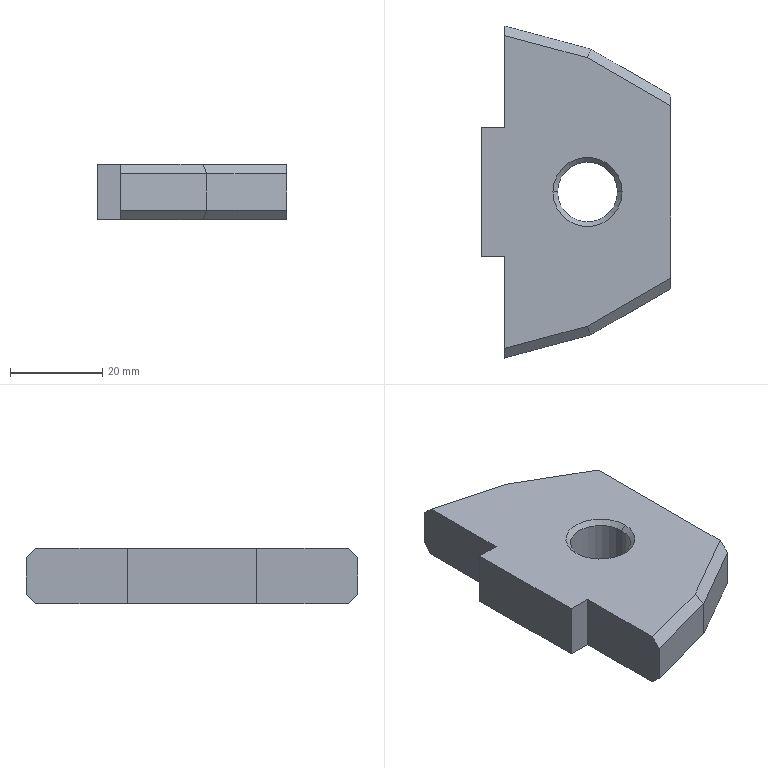Part | SolidWorks | features Chamfer 2, Extrusion 1 | 1 solid | 26 faces | box 41 x 72 x 12 mm | volume 25554 mm3 | plane 20 | cone 4 | cylinder 2 | commonest cylinder face diameters 13 x2
STEP:
#1=CARTESIAN_POINT('',(-6.5,0.,5.));
#2=VERTEX_POINT('',#1);
#3=CARTESIAN_POINT('',(6.5,0.,5.));
#4=VERTEX_POINT('',#3);
#5=CARTESIAN_POINT('',(0.,0.,5.));
#6=DIRECTION('',(0.,0.,1.));
#7=DIRECTION('',(-1.,0.,0.));
#8=AXIS2_PLACEMENT_3D('',#5,#6,#7);
#9=CIRCLE('',#8,6.5);
#10=EDGE_CURVE('',#2,#4,#9,.T.);
#11=ORIENTED_EDGE('',*,*,#10,.F.);
#12=CARTESIAN_POINT('',(-7.5,0.,6.));
#13=VERTEX_POINT('',#12);
#14=CARTESIAN_POINT('',(-7.5,0.,6.));
#15=DIRECTION('',(-0.7071,0.,0.7071));
#16=VECTOR('',#15,1000.);
#17=LINE('',#14,#16);
#18=EDGE_CURVE('',#2,#13,#17,.T.);
#19=ORIENTED_EDGE('',*,*,#18,.T.);
#20=CARTESIAN_POINT('',(7.5,0.,6.));
#21=VERTEX_POINT('',#20);
#22=CARTESIAN_POINT('',(0.,0.,6.));
#23=DIRECTION('',(0.,0.,-1.));
#24=DIRECTION('',(-1.,0.,0.));
#25=AXIS2_PLACEMENT_3D('',#22,#23,#24);
#26=CIRCLE('',#25,7.5);
#27=EDGE_CURVE('',#21,#13,#26,.T.);
#28=ORIENTED_EDGE('',*,*,#27,.F.);
#29=CARTESIAN_POINT('',(7.5,0.,6.));
#30=DIRECTION('',(0.7071,0.,0.7071));
#31=VECTOR('',#30,1000.);
#32=LINE('',#29,#31);
#33=EDGE_CURVE('',#4,#21,#32,.T.);
#34=ORIENTED_EDGE('',*,*,#33,.F.);
#35=EDGE_LOOP('',(#11,#19,#28,#34));
#36=FACE_OUTER_BOUND('',#35,.T.);
#37=CARTESIAN_POINT('',(0.,0.,6.));
#38=DIRECTION('',(0.,0.,1.));
#39=DIRECTION('',(1.,0.,0.));
#40=AXIS2_PLACEMENT_3D('',#37,#38,#39);
#41=CONICAL_SURFACE('',#40,7.5,0.7854);
#42=ADVANCED_FACE('',(#36),#41,.F.);
#43=CARTESIAN_POINT('',(6.5,0.,-5.));
#44=VERTEX_POINT('',#43);
#45=CARTESIAN_POINT('',(-6.5,0.,-5.));
#46=VERTEX_POINT('',#45);
#47=CARTESIAN_POINT('',(0.,0.,-5.));
#48=DIRECTION('',(0.,0.,-1.));
#49=DIRECTION('',(-1.,0.,0.));
#50=AXIS2_PLACEMENT_3D('',#47,#48,#49);
#51=CIRCLE('',#50,6.5);
#52=EDGE_CURVE('',#44,#46,#51,.T.);
#53=ORIENTED_EDGE('',*,*,#52,.F.);
#54=CARTESIAN_POINT('',(7.5,0.,-6.));
#55=VERTEX_POINT('',#54);
#56=CARTESIAN_POINT('',(6.5,0.,-5.));
#57=DIRECTION('',(0.7071,0.,-0.7071));
#58=VECTOR('',#57,1000.);
#59=LINE('',#56,#58);
#60=EDGE_CURVE('',#44,#55,#59,.T.);
#61=ORIENTED_EDGE('',*,*,#60,.T.);
#62=CARTESIAN_POINT('',(-7.5,0.,-6.));
#63=VERTEX_POINT('',#62);
#64=CARTESIAN_POINT('',(0.,0.,-6.));
#65=DIRECTION('',(0.,0.,1.));
#66=DIRECTION('',(-1.,0.,0.));
#67=AXIS2_PLACEMENT_3D('',#64,#65,#66);
#68=CIRCLE('',#67,7.5);
#69=EDGE_CURVE('',#63,#55,#68,.T.);
#70=ORIENTED_EDGE('',*,*,#69,.F.);
#71=CARTESIAN_POINT('',(-6.5,0.,-5.));
#72=DIRECTION('',(-0.7071,0.,-0.7071));
#73=VECTOR('',#72,1000.);
#74=LINE('',#71,#73);
#75=EDGE_CURVE('',#46,#63,#74,.T.);
#76=ORIENTED_EDGE('',*,*,#75,.F.);
#77=EDGE_LOOP('',(#53,#61,#70,#76));
#78=FACE_OUTER_BOUND('',#77,.T.);
#79=CARTESIAN_POINT('',(0.,0.,-5.));
#80=DIRECTION('',(0.,0.,-1.));
#81=DIRECTION('',(-1.,0.,0.));
#82=AXIS2_PLACEMENT_3D('',#79,#80,#81);
#83=CONICAL_SURFACE('',#82,6.5,0.7854);
#84=ADVANCED_FACE('',(#78),#83,.F.);
#85=ORIENTED_EDGE('',*,*,#10,.T.);
#86=CARTESIAN_POINT('',(6.5,0.,6.));
#87=DIRECTION('',(0.,0.,-1.));
#88=VECTOR('',#87,1000.);
#89=LINE('',#86,#88);
#90=EDGE_CURVE('',#4,#44,#89,.T.);
#91=ORIENTED_EDGE('',*,*,#90,.T.);
#92=ORIENTED_EDGE('',*,*,#52,.T.);
#93=CARTESIAN_POINT('',(-6.5,0.,6.));
#94=DIRECTION('',(0.,0.,-1.));
#95=VECTOR('',#94,1000.);
#96=LINE('',#93,#95);
#97=EDGE_CURVE('',#2,#46,#96,.T.);
#98=ORIENTED_EDGE('',*,*,#97,.F.);
#99=EDGE_LOOP('',(#85,#91,#92,#98));
#100=FACE_OUTER_BOUND('',#99,.T.);
#101=CARTESIAN_POINT('',(0.,0.,6.));
#102=DIRECTION('',(0.,0.,-1.));
#103=DIRECTION('',(-1.,0.,0.));
#104=AXIS2_PLACEMENT_3D('',#101,#102,#103);
#105=CYLINDRICAL_SURFACE('',#104,6.5);
#106=ADVANCED_FACE('',(#100),#105,.F.);
#107=CARTESIAN_POINT('',(-18.,36.,4.));
#108=VERTEX_POINT('',#107);
#109=CARTESIAN_POINT('',(-18.,36.,-4.));
#110=VERTEX_POINT('',#109);
#111=CARTESIAN_POINT('',(-18.,36.,6.));
#112=DIRECTION('',(0.,0.,-1.));
#113=VECTOR('',#112,1000.);
#114=LINE('',#111,#113);
#115=EDGE_CURVE('',#108,#110,#114,.T.);
#116=ORIENTED_EDGE('',*,*,#115,.T.);
#117=CARTESIAN_POINT('',(-18.,33.929,-6.));
#118=VERTEX_POINT('',#117);
#119=CARTESIAN_POINT('',(-18.,29.616,-10.167));
#120=DIRECTION('',(0.,-0.7193,-0.6947));
#121=VECTOR('',#120,1000.);
#122=LINE('',#119,#121);
#123=EDGE_CURVE('',#110,#118,#122,.T.);
#124=ORIENTED_EDGE('',*,*,#123,.T.);
#125=CARTESIAN_POINT('',(-18.,14.,-6.));
#126=VERTEX_POINT('',#125);
#127=CARTESIAN_POINT('',(-18.,14.,-6.));
#128=DIRECTION('',(0.,1.,0.));
#129=VECTOR('',#128,1000.);
#130=LINE('',#127,#129);
#131=EDGE_CURVE('',#126,#118,#130,.T.);
#132=ORIENTED_EDGE('',*,*,#131,.F.);
#133=CARTESIAN_POINT('',(-18.,14.,6.));
#134=VERTEX_POINT('',#133);
#135=CARTESIAN_POINT('',(-18.,14.,6.));
#136=DIRECTION('',(0.,0.,-1.));
#137=VECTOR('',#136,1000.);
#138=LINE('',#135,#137);
#139=EDGE_CURVE('',#134,#126,#138,.T.);
#140=ORIENTED_EDGE('',*,*,#139,.F.);
#141=CARTESIAN_POINT('',(-18.,33.929,6.));
#142=VERTEX_POINT('',#141);
#143=CARTESIAN_POINT('',(-18.,14.,6.));
#144=DIRECTION('',(0.,1.,0.));
#145=VECTOR('',#144,1000.);
#146=LINE('',#143,#145);
#147=EDGE_CURVE('',#134,#142,#146,.T.);
#148=ORIENTED_EDGE('',*,*,#147,.T.);
#149=CARTESIAN_POINT('',(-18.,23.619,15.959));
#150=DIRECTION('',(0.,0.7193,-0.6947));
#151=VECTOR('',#150,1000.);
#152=LINE('',#149,#151);
#153=EDGE_CURVE('',#142,#108,#152,.T.);
#154=ORIENTED_EDGE('',*,*,#153,.T.);
#155=EDGE_LOOP('',(#116,#124,#132,#140,#148,#154));
#156=FACE_OUTER_BOUND('',#155,.T.);
#157=CARTESIAN_POINT('',(-18.,14.,6.));
#158=DIRECTION('',(-1.,0.,0.));
#159=DIRECTION('',(0.,0.,1.));
#160=AXIS2_PLACEMENT_3D('',#157,#158,#159);
#161=PLANE('',#160);
#162=ADVANCED_FACE('',(#156),#161,.T.);
#163=CARTESIAN_POINT('',(-23.,14.,-6.));
#164=VERTEX_POINT('',#163);
#165=CARTESIAN_POINT('',(-23.,14.,-6.));
#166=DIRECTION('',(1.,0.,0.));
#167=VECTOR('',#166,1000.);
#168=LINE('',#165,#167);
#169=EDGE_CURVE('',#164,#126,#168,.T.);
#170=ORIENTED_EDGE('',*,*,#169,.F.);
#171=CARTESIAN_POINT('',(-23.,14.,6.));
#172=VERTEX_POINT('',#171);
#173=CARTESIAN_POINT('',(-23.,14.,6.));
#174=DIRECTION('',(0.,0.,-1.));
#175=VECTOR('',#174,1000.);
#176=LINE('',#173,#175);
#177=EDGE_CURVE('',#172,#164,#176,.T.);
#178=ORIENTED_EDGE('',*,*,#177,.F.);
#179=CARTESIAN_POINT('',(-23.,14.,6.));
#180=DIRECTION('',(1.,0.,0.));
#181=VECTOR('',#180,1000.);
#182=LINE('',#179,#181);
#183=EDGE_CURVE('',#172,#134,#182,.T.);
#184=ORIENTED_EDGE('',*,*,#183,.T.);
#185=ORIENTED_EDGE('',*,*,#139,.T.);
#186=EDGE_LOOP('',(#170,#178,#184,#185));
#187=FACE_OUTER_BOUND('',#186,.T.);
#188=CARTESIAN_POINT('',(-23.,14.,6.));
#189=DIRECTION('',(0.,1.,0.));
#190=DIRECTION('',(0.,0.,1.));
#191=AXIS2_PLACEMENT_3D('',#188,#189,#190);
#192=PLANE('',#191);
#193=ADVANCED_FACE('',(#187),#192,.T.);
#194=CARTESIAN_POINT('',(-23.,-14.,-6.));
#195=VERTEX_POINT('',#194);
#196=CARTESIAN_POINT('',(-23.,-14.,-6.));
#197=DIRECTION('',(0.,1.,0.));
#198=VECTOR('',#197,1000.);
#199=LINE('',#196,#198);
#200=EDGE_CURVE('',#195,#164,#199,.T.);
#201=ORIENTED_EDGE('',*,*,#200,.F.);
#202=CARTESIAN_POINT('',(-23.,-14.,6.));
#203=VERTEX_POINT('',#202);
#204=CARTESIAN_POINT('',(-23.,-14.,6.));
#205=DIRECTION('',(0.,0.,-1.));
#206=VECTOR('',#205,1000.);
#207=LINE('',#204,#206);
#208=EDGE_CURVE('',#203,#195,#207,.T.);
#209=ORIENTED_EDGE('',*,*,#208,.F.);
#210=CARTESIAN_POINT('',(-23.,-14.,6.));
#211=DIRECTION('',(0.,1.,0.));
#212=VECTOR('',#211,1000.);
#213=LINE('',#210,#212);
#214=EDGE_CURVE('',#203,#172,#213,.T.);
#215=ORIENTED_EDGE('',*,*,#214,.T.);
#216=ORIENTED_EDGE('',*,*,#177,.T.);
#217=EDGE_LOOP('',(#201,#209,#215,#216));
#218=FACE_OUTER_BOUND('',#217,.T.);
#219=CARTESIAN_POINT('',(-23.,-14.,6.));
#220=DIRECTION('',(-1.,0.,0.));
#221=DIRECTION('',(0.,0.,1.));
#222=AXIS2_PLACEMENT_3D('',#219,#220,#221);
#223=PLANE('',#222);
#224=ADVANCED_FACE('',(#218),#223,.T.);
#225=CARTESIAN_POINT('',(-18.,-14.,-6.));
#226=VERTEX_POINT('',#225);
#227=CARTESIAN_POINT('',(-23.,-14.,-6.));
#228=DIRECTION('',(1.,0.,0.));
#229=VECTOR('',#228,1000.);
#230=LINE('',#227,#229);
#231=EDGE_CURVE('',#195,#226,#230,.T.);
#232=ORIENTED_EDGE('',*,*,#231,.T.);
#233=CARTESIAN_POINT('',(-18.,-14.,6.));
#234=VERTEX_POINT('',#233);
#235=CARTESIAN_POINT('',(-18.,-14.,6.));
#236=DIRECTION('',(0.,0.,-1.));
#237=VECTOR('',#236,1000.);
#238=LINE('',#235,#237);
#239=EDGE_CURVE('',#234,#226,#238,.T.);
#240=ORIENTED_EDGE('',*,*,#239,.F.);
#241=CARTESIAN_POINT('',(-23.,-14.,6.));
#242=DIRECTION('',(1.,0.,0.));
#243=VECTOR('',#242,1000.);
#244=LINE('',#241,#243);
#245=EDGE_CURVE('',#203,#234,#244,.T.);
#246=ORIENTED_EDGE('',*,*,#245,.F.);
#247=ORIENTED_EDGE('',*,*,#208,.T.);
#248=EDGE_LOOP('',(#232,#240,#246,#247));
#249=FACE_OUTER_BOUND('',#248,.T.);
#250=CARTESIAN_POINT('',(-23.,-14.,6.));
#251=DIRECTION('',(0.,1.,0.));
#252=DIRECTION('',(0.,0.,1.));
#253=AXIS2_PLACEMENT_3D('',#250,#251,#252);
#254=PLANE('',#253);
#255=ADVANCED_FACE('',(#249),#254,.F.);
#256=CARTESIAN_POINT('',(-18.,-33.929,-6.));
#257=VERTEX_POINT('',#256);
#258=CARTESIAN_POINT('',(-18.,-14.,-6.));
#259=DIRECTION('',(0.,-1.,0.));
#260=VECTOR('',#259,1000.);
#261=LINE('',#258,#260);
#262=EDGE_CURVE('',#226,#257,#261,.T.);
#263=ORIENTED_EDGE('',*,*,#262,.T.);
#264=CARTESIAN_POINT('',(-18.,-36.,-4.));
#265=VERTEX_POINT('',#264);
#266=CARTESIAN_POINT('',(-18.,-36.,-4.));
#267=DIRECTION('',(0.,-0.7193,0.6947));
#268=VECTOR('',#267,1000.);
#269=LINE('',#266,#268);
#270=EDGE_CURVE('',#257,#265,#269,.T.);
#271=ORIENTED_EDGE('',*,*,#270,.T.);
#272=CARTESIAN_POINT('',(-18.,-36.,4.));
#273=VERTEX_POINT('',#272);
#274=CARTESIAN_POINT('',(-18.,-36.,6.));
#275=DIRECTION('',(0.,0.,-1.));
#276=VECTOR('',#275,1000.);
#277=LINE('',#274,#276);
#278=EDGE_CURVE('',#273,#265,#277,.T.);
#279=ORIENTED_EDGE('',*,*,#278,.F.);
#280=CARTESIAN_POINT('',(-18.,-33.929,6.));
#281=VERTEX_POINT('',#280);
#282=CARTESIAN_POINT('',(-18.,-30.426,9.384));
#283=DIRECTION('',(0.,0.7193,0.6947));
#284=VECTOR('',#283,1000.);
#285=LINE('',#282,#284);
#286=EDGE_CURVE('',#273,#281,#285,.T.);
#287=ORIENTED_EDGE('',*,*,#286,.T.);
#288=CARTESIAN_POINT('',(-18.,-14.,6.));
#289=DIRECTION('',(0.,-1.,0.));
#290=VECTOR('',#289,1000.);
#291=LINE('',#288,#290);
#292=EDGE_CURVE('',#234,#281,#291,.T.);
#293=ORIENTED_EDGE('',*,*,#292,.F.);
#294=ORIENTED_EDGE('',*,*,#239,.T.);
#295=EDGE_LOOP('',(#263,#271,#279,#287,#293,#294));
#296=FACE_OUTER_BOUND('',#295,.T.);
#297=CARTESIAN_POINT('',(-18.,-14.,6.));
#298=DIRECTION('',(1.,0.,0.));
#299=DIRECTION('',(0.,1.,0.));
#300=AXIS2_PLACEMENT_3D('',#297,#298,#299);
#301=PLANE('',#300);
#302=ADVANCED_FACE('',(#296),#301,.F.);
#303=ORIENTED_EDGE('',*,*,#278,.T.);
#304=CARTESIAN_POINT('',(0.6962,-30.99,-4.));
#305=VERTEX_POINT('',#304);
#306=CARTESIAN_POINT('',(0.6962,-30.99,-4.));
#307=DIRECTION('',(0.9659,0.2588,0.));
#308=VECTOR('',#307,1000.);
#309=LINE('',#306,#308);
#310=EDGE_CURVE('',#265,#305,#309,.T.);
#311=ORIENTED_EDGE('',*,*,#310,.T.);
#312=CARTESIAN_POINT('',(0.6962,-30.99,4.));
#313=VERTEX_POINT('',#312);
#314=CARTESIAN_POINT('',(0.6962,-30.99,6.));
#315=DIRECTION('',(0.,0.,-1.));
#316=VECTOR('',#315,1000.);
#317=LINE('',#314,#316);
#318=EDGE_CURVE('',#313,#305,#317,.T.);
#319=ORIENTED_EDGE('',*,*,#318,.F.);
#320=CARTESIAN_POINT('',(-18.,-36.,4.));
#321=DIRECTION('',(-0.9659,-0.2588,0.));
#322=VECTOR('',#321,1000.);
#323=LINE('',#320,#322);
#324=EDGE_CURVE('',#313,#273,#323,.T.);
#325=ORIENTED_EDGE('',*,*,#324,.T.);
#326=EDGE_LOOP('',(#303,#311,#319,#325));
#327=FACE_OUTER_BOUND('',#326,.T.);
#328=CARTESIAN_POINT('',(-18.,-36.,6.));
#329=DIRECTION('',(-0.2588,0.9659,0.));
#330=DIRECTION('',(-0.9659,-0.2588,0.));
#331=AXIS2_PLACEMENT_3D('',#328,#329,#330);
#332=PLANE('',#331);
#333=ADVANCED_FACE('',(#327),#332,.F.);
#334=ORIENTED_EDGE('',*,*,#318,.T.);
#335=CARTESIAN_POINT('',(18.,-21.,-4.));
#336=VERTEX_POINT('',#335);
#337=CARTESIAN_POINT('',(18.,-21.,-4.));
#338=DIRECTION('',(0.866,0.5,0.));
#339=VECTOR('',#338,1000.);
#340=LINE('',#337,#339);
#341=EDGE_CURVE('',#305,#336,#340,.T.);
#342=ORIENTED_EDGE('',*,*,#341,.T.);
#343=CARTESIAN_POINT('',(18.,-21.,4.));
#344=VERTEX_POINT('',#343);
#345=CARTESIAN_POINT('',(18.,-21.,6.));
#346=DIRECTION('',(0.,0.,-1.));
#347=VECTOR('',#346,1000.);
#348=LINE('',#345,#347);
#349=EDGE_CURVE('',#344,#336,#348,.T.);
#350=ORIENTED_EDGE('',*,*,#349,.F.);
#351=CARTESIAN_POINT('',(0.6962,-30.99,4.));
#352=DIRECTION('',(-0.866,-0.5,0.));
#353=VECTOR('',#352,1000.);
#354=LINE('',#351,#353);
#355=EDGE_CURVE('',#344,#313,#354,.T.);
#356=ORIENTED_EDGE('',*,*,#355,.T.);
#357=EDGE_LOOP('',(#334,#342,#350,#356));
#358=FACE_OUTER_BOUND('',#357,.T.);
#359=CARTESIAN_POINT('',(0.6962,-30.99,6.));
#360=DIRECTION('',(-0.5,0.866,0.));
#361=DIRECTION('',(-0.866,-0.5,0.));
#362=AXIS2_PLACEMENT_3D('',#359,#360,#361);
#363=PLANE('',#362);
#364=ADVANCED_FACE('',(#358),#363,.F.);
#365=ORIENTED_EDGE('',*,*,#349,.T.);
#366=CARTESIAN_POINT('',(18.,-18.691,-6.));
#367=VERTEX_POINT('',#366);
#368=CARTESIAN_POINT('',(18.,-1.949,-20.499));
#369=DIRECTION('',(0.,0.7559,-0.6547));
#370=VECTOR('',#369,1000.);
#371=LINE('',#368,#370);
#372=EDGE_CURVE('',#336,#367,#371,.T.);
#373=ORIENTED_EDGE('',*,*,#372,.T.);
#374=CARTESIAN_POINT('',(18.,18.691,-6.));
#375=VERTEX_POINT('',#374);
#376=CARTESIAN_POINT('',(18.,21.,-6.));
#377=DIRECTION('',(0.,-1.,0.));
#378=VECTOR('',#377,1000.);
#379=LINE('',#376,#378);
#380=EDGE_CURVE('',#375,#367,#379,.T.);
#381=ORIENTED_EDGE('',*,*,#380,.F.);
#382=CARTESIAN_POINT('',(18.,21.,-4.));
#383=VERTEX_POINT('',#382);
#384=CARTESIAN_POINT('',(18.,25.949,0.2857));
#385=DIRECTION('',(0.,0.7559,0.6547));
#386=VECTOR('',#385,1000.);
#387=LINE('',#384,#386);
#388=EDGE_CURVE('',#375,#383,#387,.T.);
#389=ORIENTED_EDGE('',*,*,#388,.T.);
#390=CARTESIAN_POINT('',(18.,21.,4.));
#391=VERTEX_POINT('',#390);
#392=CARTESIAN_POINT('',(18.,21.,6.));
#393=DIRECTION('',(0.,0.,-1.));
#394=VECTOR('',#393,1000.);
#395=LINE('',#392,#394);
#396=EDGE_CURVE('',#391,#383,#395,.T.);
#397=ORIENTED_EDGE('',*,*,#396,.F.);
#398=CARTESIAN_POINT('',(18.,18.691,6.));
#399=VERTEX_POINT('',#398);
#400=CARTESIAN_POINT('',(18.,20.01,4.857));
#401=DIRECTION('',(0.,-0.7559,0.6547));
#402=VECTOR('',#401,1000.);
#403=LINE('',#400,#402);
#404=EDGE_CURVE('',#391,#399,#403,.T.);
#405=ORIENTED_EDGE('',*,*,#404,.T.);
#406=CARTESIAN_POINT('',(18.,-18.691,6.));
#407=VERTEX_POINT('',#406);
#408=CARTESIAN_POINT('',(18.,21.,6.));
#409=DIRECTION('',(0.,-1.,0.));
#410=VECTOR('',#409,1000.);
#411=LINE('',#408,#410);
#412=EDGE_CURVE('',#399,#407,#411,.T.);
#413=ORIENTED_EDGE('',*,*,#412,.T.);
#414=CARTESIAN_POINT('',(18.,3.99,25.642));
#415=DIRECTION('',(0.,-0.7559,-0.6547));
#416=VECTOR('',#415,1000.);
#417=LINE('',#414,#416);
#418=EDGE_CURVE('',#407,#344,#417,.T.);
#419=ORIENTED_EDGE('',*,*,#418,.T.);
#420=EDGE_LOOP('',(#365,#373,#381,#389,#397,#405,#413,#419));
#421=FACE_OUTER_BOUND('',#420,.T.);
#422=CARTESIAN_POINT('',(18.,21.,6.));
#423=DIRECTION('',(1.,0.,0.));
#424=DIRECTION('',(0.,1.,0.));
#425=AXIS2_PLACEMENT_3D('',#422,#423,#424);
#426=PLANE('',#425);
#427=ADVANCED_FACE('',(#421),#426,.T.);
#428=ORIENTED_EDGE('',*,*,#396,.T.);
#429=CARTESIAN_POINT('',(0.6962,30.99,-4.));
#430=VERTEX_POINT('',#429);
#431=CARTESIAN_POINT('',(0.6962,30.99,-4.));
#432=DIRECTION('',(-0.866,0.5,0.));
#433=VECTOR('',#432,1000.);
#434=LINE('',#431,#433);
#435=EDGE_CURVE('',#383,#430,#434,.T.);
#436=ORIENTED_EDGE('',*,*,#435,.T.);
#437=CARTESIAN_POINT('',(0.6962,30.99,4.));
#438=VERTEX_POINT('',#437);
#439=CARTESIAN_POINT('',(0.6962,30.99,6.));
#440=DIRECTION('',(0.,0.,-1.));
#441=VECTOR('',#440,1000.);
#442=LINE('',#439,#441);
#443=EDGE_CURVE('',#438,#430,#442,.T.);
#444=ORIENTED_EDGE('',*,*,#443,.F.);
#445=CARTESIAN_POINT('',(18.,21.,4.));
#446=DIRECTION('',(0.866,-0.5,0.));
#447=VECTOR('',#446,1000.);
#448=LINE('',#445,#447);
#449=EDGE_CURVE('',#438,#391,#448,.T.);
#450=ORIENTED_EDGE('',*,*,#449,.T.);
#451=EDGE_LOOP('',(#428,#436,#444,#450));
#452=FACE_OUTER_BOUND('',#451,.T.);
#453=CARTESIAN_POINT('',(0.6962,30.99,6.));
#454=DIRECTION('',(0.5,0.866,0.));
#455=DIRECTION('',(-0.866,0.5,0.));
#456=AXIS2_PLACEMENT_3D('',#453,#454,#455);
#457=PLANE('',#456);
#458=ADVANCED_FACE('',(#452),#457,.T.);
#459=ORIENTED_EDGE('',*,*,#443,.T.);
#460=CARTESIAN_POINT('',(-18.,36.,-4.));
#461=DIRECTION('',(-0.9659,0.2588,0.));
#462=VECTOR('',#461,1000.);
#463=LINE('',#460,#462);
#464=EDGE_CURVE('',#430,#110,#463,.T.);
#465=ORIENTED_EDGE('',*,*,#464,.T.);
#466=ORIENTED_EDGE('',*,*,#115,.F.);
#467=CARTESIAN_POINT('',(0.6962,30.99,4.));
#468=DIRECTION('',(0.9659,-0.2588,0.));
#469=VECTOR('',#468,1000.);
#470=LINE('',#467,#469);
#471=EDGE_CURVE('',#108,#438,#470,.T.);
#472=ORIENTED_EDGE('',*,*,#471,.T.);
#473=EDGE_LOOP('',(#459,#465,#466,#472));
#474=FACE_OUTER_BOUND('',#473,.T.);
#475=CARTESIAN_POINT('',(-18.,36.,6.));
#476=DIRECTION('',(0.2588,0.9659,0.));
#477=DIRECTION('',(-0.9659,0.2588,0.));
#478=AXIS2_PLACEMENT_3D('',#475,#476,#477);
#479=PLANE('',#478);
#480=ADVANCED_FACE('',(#474),#479,.T.);
#481=ORIENTED_EDGE('',*,*,#27,.T.);
#482=CARTESIAN_POINT('',(0.,0.,6.));
#483=DIRECTION('',(0.,0.,-1.));
#484=DIRECTION('',(-1.,0.,0.));
#485=AXIS2_PLACEMENT_3D('',#482,#483,#484);
#486=CIRCLE('',#485,7.5);
#487=EDGE_CURVE('',#13,#21,#486,.T.);
#488=ORIENTED_EDGE('',*,*,#487,.T.);
#489=EDGE_LOOP('',(#481,#488));
#490=FACE_BOUND('',#489,.T.);
#491=CARTESIAN_POINT('',(-0.07582,-29.127,6.));
#492=VERTEX_POINT('',#491);
#493=CARTESIAN_POINT('',(7.277,-27.157,6.));
#494=DIRECTION('',(0.9659,0.2588,0.));
#495=VECTOR('',#494,1000.);
#496=LINE('',#493,#495);
#497=EDGE_CURVE('',#281,#492,#496,.T.);
#498=ORIENTED_EDGE('',*,*,#497,.T.);
#499=CARTESIAN_POINT('',(12.593,-21.812,6.));
#500=DIRECTION('',(0.866,0.5,0.));
#501=VECTOR('',#500,1000.);
#502=LINE('',#499,#501);
#503=EDGE_CURVE('',#492,#407,#502,.T.);
#504=ORIENTED_EDGE('',*,*,#503,.T.);
#505=ORIENTED_EDGE('',*,*,#412,.F.);
#506=CARTESIAN_POINT('',(-0.07582,29.127,6.));
#507=VERTEX_POINT('',#506);
#508=CARTESIAN_POINT('',(-0.3038,29.258,6.));
#509=DIRECTION('',(-0.866,0.5,0.));
#510=VECTOR('',#509,1000.);
#511=LINE('',#508,#510);
#512=EDGE_CURVE('',#399,#507,#511,.T.);
#513=ORIENTED_EDGE('',*,*,#512,.T.);
#514=CARTESIAN_POINT('',(-18.518,34.068,6.));
#515=DIRECTION('',(-0.9659,0.2588,0.));
#516=VECTOR('',#515,1000.);
#517=LINE('',#514,#516);
#518=EDGE_CURVE('',#507,#142,#517,.T.);
#519=ORIENTED_EDGE('',*,*,#518,.T.);
#520=ORIENTED_EDGE('',*,*,#147,.F.);
#521=ORIENTED_EDGE('',*,*,#183,.F.);
#522=ORIENTED_EDGE('',*,*,#214,.F.);
#523=ORIENTED_EDGE('',*,*,#245,.T.);
#524=ORIENTED_EDGE('',*,*,#292,.T.);
#525=EDGE_LOOP('',(#498,#504,#505,#513,#519,#520,#521,#522,#523,#524));
#526=FACE_OUTER_BOUND('',#525,.T.);
#527=CARTESIAN_POINT('',(0.,0.,6.));
#528=DIRECTION('',(0.,0.,-1.));
#529=DIRECTION('',(-1.,0.,0.));
#530=AXIS2_PLACEMENT_3D('',#527,#528,#529);
#531=PLANE('',#530);
#532=ADVANCED_FACE('',(#490,#526),#531,.F.);
#533=ORIENTED_EDGE('',*,*,#69,.T.);
#534=CARTESIAN_POINT('',(0.,0.,-6.));
#535=DIRECTION('',(0.,0.,1.));
#536=DIRECTION('',(-1.,0.,0.));
#537=AXIS2_PLACEMENT_3D('',#534,#535,#536);
#538=CIRCLE('',#537,7.5);
#539=EDGE_CURVE('',#55,#63,#538,.T.);
#540=ORIENTED_EDGE('',*,*,#539,.T.);
#541=EDGE_LOOP('',(#533,#540));
#542=FACE_BOUND('',#541,.T.);
#543=ORIENTED_EDGE('',*,*,#380,.T.);
#544=CARTESIAN_POINT('',(-0.07582,-29.127,-6.));
#545=VERTEX_POINT('',#544);
#546=CARTESIAN_POINT('',(-0.3038,-29.258,-6.));
#547=DIRECTION('',(-0.866,-0.5,0.));
#548=VECTOR('',#547,1000.);
#549=LINE('',#546,#548);
#550=EDGE_CURVE('',#367,#545,#549,.T.);
#551=ORIENTED_EDGE('',*,*,#550,.T.);
#552=CARTESIAN_POINT('',(-18.518,-34.068,-6.));
#553=DIRECTION('',(-0.9659,-0.2588,0.));
#554=VECTOR('',#553,1000.);
#555=LINE('',#552,#554);
#556=EDGE_CURVE('',#545,#257,#555,.T.);
#557=ORIENTED_EDGE('',*,*,#556,.T.);
#558=ORIENTED_EDGE('',*,*,#262,.F.);
#559=ORIENTED_EDGE('',*,*,#231,.F.);
#560=ORIENTED_EDGE('',*,*,#200,.T.);
#561=ORIENTED_EDGE('',*,*,#169,.T.);
#562=ORIENTED_EDGE('',*,*,#131,.T.);
#563=CARTESIAN_POINT('',(-0.07582,29.127,-6.));
#564=VERTEX_POINT('',#563);
#565=CARTESIAN_POINT('',(7.277,27.157,-6.));
#566=DIRECTION('',(0.9659,-0.2588,0.));
#567=VECTOR('',#566,1000.);
#568=LINE('',#565,#567);
#569=EDGE_CURVE('',#118,#564,#568,.T.);
#570=ORIENTED_EDGE('',*,*,#569,.T.);
#571=CARTESIAN_POINT('',(12.593,21.812,-6.));
#572=DIRECTION('',(0.866,-0.5,0.));
#573=VECTOR('',#572,1000.);
#574=LINE('',#571,#573);
#575=EDGE_CURVE('',#564,#375,#574,.T.);
#576=ORIENTED_EDGE('',*,*,#575,.T.);
#577=EDGE_LOOP('',(#543,#551,#557,#558,#559,#560,#561,#562,#570,#576));
#578=FACE_OUTER_BOUND('',#577,.T.);
#579=CARTESIAN_POINT('',(0.,0.,-6.));
#580=DIRECTION('',(0.,0.,-1.));
#581=DIRECTION('',(-1.,0.,0.));
#582=AXIS2_PLACEMENT_3D('',#579,#580,#581);
#583=PLANE('',#582);
#584=ADVANCED_FACE('',(#542,#578),#583,.T.);
#585=ORIENTED_EDGE('',*,*,#90,.F.);
#586=CARTESIAN_POINT('',(0.,0.,5.));
#587=DIRECTION('',(0.,0.,1.));
#588=DIRECTION('',(-1.,0.,0.));
#589=AXIS2_PLACEMENT_3D('',#586,#587,#588);
#590=CIRCLE('',#589,6.5);
#591=EDGE_CURVE('',#4,#2,#590,.T.);
#592=ORIENTED_EDGE('',*,*,#591,.T.);
#593=ORIENTED_EDGE('',*,*,#97,.T.);
#594=CARTESIAN_POINT('',(0.,0.,-5.));
#595=DIRECTION('',(0.,0.,-1.));
#596=DIRECTION('',(-1.,0.,0.));
#597=AXIS2_PLACEMENT_3D('',#594,#595,#596);
#598=CIRCLE('',#597,6.5);
#599=EDGE_CURVE('',#46,#44,#598,.T.);
#600=ORIENTED_EDGE('',*,*,#599,.T.);
#601=EDGE_LOOP('',(#585,#592,#593,#600));
#602=FACE_OUTER_BOUND('',#601,.T.);
#603=CARTESIAN_POINT('',(0.,0.,6.));
#604=DIRECTION('',(0.,0.,-1.));
#605=DIRECTION('',(-1.,0.,0.));
#606=AXIS2_PLACEMENT_3D('',#603,#604,#605);
#607=CYLINDRICAL_SURFACE('',#606,6.5);
#608=ADVANCED_FACE('',(#602),#607,.F.);
#609=ORIENTED_EDGE('',*,*,#270,.F.);
#610=ORIENTED_EDGE('',*,*,#556,.F.);
#611=CARTESIAN_POINT('',(0.2086,-29.813,-5.263));
#612=DIRECTION('',(-0.2718,0.6561,-0.7041));
#613=VECTOR('',#612,1000.);
#614=LINE('',#611,#613);
#615=EDGE_CURVE('',#305,#545,#614,.T.);
#616=ORIENTED_EDGE('',*,*,#615,.F.);
#617=ORIENTED_EDGE('',*,*,#310,.F.);
#618=EDGE_LOOP('',(#609,#610,#616,#617));
#619=FACE_OUTER_BOUND('',#618,.T.);
#620=CARTESIAN_POINT('',(-18.,-36.,-4.));
#621=DIRECTION('',(0.183,-0.683,-0.7071));
#622=DIRECTION('',(-0.9659,-0.2588,0.));
#623=AXIS2_PLACEMENT_3D('',#620,#621,#622);
#624=PLANE('',#623);
#625=ADVANCED_FACE('',(#619),#624,.T.);
#626=ORIENTED_EDGE('',*,*,#615,.T.);
#627=ORIENTED_EDGE('',*,*,#550,.F.);
#628=ORIENTED_EDGE('',*,*,#372,.F.);
#629=ORIENTED_EDGE('',*,*,#341,.F.);
#630=EDGE_LOOP('',(#626,#627,#628,#629));
#631=FACE_OUTER_BOUND('',#630,.T.);
#632=CARTESIAN_POINT('',(0.6962,-30.99,-4.));
#633=DIRECTION('',(0.3536,-0.6124,-0.7071));
#634=DIRECTION('',(-0.866,-0.5,0.));
#635=AXIS2_PLACEMENT_3D('',#632,#633,#634);
#636=PLANE('',#635);
#637=ADVANCED_FACE('',(#631),#636,.T.);
#638=ORIENTED_EDGE('',*,*,#286,.F.);
#639=ORIENTED_EDGE('',*,*,#324,.F.);
#640=CARTESIAN_POINT('',(0.1159,-29.59,5.503));
#641=DIRECTION('',(0.2718,-0.6561,-0.7041));
#642=VECTOR('',#641,1000.);
#643=LINE('',#640,#642);
#644=EDGE_CURVE('',#492,#313,#643,.T.);
#645=ORIENTED_EDGE('',*,*,#644,.F.);
#646=ORIENTED_EDGE('',*,*,#497,.F.);
#647=EDGE_LOOP('',(#638,#639,#645,#646));
#648=FACE_OUTER_BOUND('',#647,.T.);
#649=CARTESIAN_POINT('',(7.277,-27.157,6.));
#650=DIRECTION('',(-0.183,0.683,-0.7071));
#651=DIRECTION('',(0.9659,0.2588,0.));
#652=AXIS2_PLACEMENT_3D('',#649,#650,#651);
#653=PLANE('',#652);
#654=ADVANCED_FACE('',(#648),#653,.F.);
#655=ORIENTED_EDGE('',*,*,#644,.T.);
#656=ORIENTED_EDGE('',*,*,#355,.F.);
#657=ORIENTED_EDGE('',*,*,#418,.F.);
#658=ORIENTED_EDGE('',*,*,#503,.F.);
#659=EDGE_LOOP('',(#655,#656,#657,#658));
#660=FACE_OUTER_BOUND('',#659,.T.);
#661=CARTESIAN_POINT('',(12.593,-21.812,6.));
#662=DIRECTION('',(-0.3536,0.6124,-0.7071));
#663=DIRECTION('',(0.866,0.5,0.));
#664=AXIS2_PLACEMENT_3D('',#661,#662,#663);
#665=PLANE('',#664);
#666=ADVANCED_FACE('',(#660),#665,.F.);
#667=ORIENTED_EDGE('',*,*,#388,.F.);
#668=ORIENTED_EDGE('',*,*,#575,.F.);
#669=CARTESIAN_POINT('',(-0.4443,28.237,-6.955));
#670=DIRECTION('',(-0.2718,-0.6561,-0.7041));
#671=VECTOR('',#670,1000.);
#672=LINE('',#669,#671);
#673=EDGE_CURVE('',#430,#564,#672,.T.);
#674=ORIENTED_EDGE('',*,*,#673,.F.);
#675=ORIENTED_EDGE('',*,*,#435,.F.);
#676=EDGE_LOOP('',(#667,#668,#674,#675));
#677=FACE_OUTER_BOUND('',#676,.T.);
#678=CARTESIAN_POINT('',(12.593,21.812,-6.));
#679=DIRECTION('',(-0.3536,-0.6124,0.7071));
#680=DIRECTION('',(0.866,-0.5,0.));
#681=AXIS2_PLACEMENT_3D('',#678,#679,#680);
#682=PLANE('',#681);
#683=ADVANCED_FACE('',(#677),#682,.F.);
#684=ORIENTED_EDGE('',*,*,#123,.F.);
#685=ORIENTED_EDGE('',*,*,#464,.F.);
#686=ORIENTED_EDGE('',*,*,#673,.T.);
#687=ORIENTED_EDGE('',*,*,#569,.F.);
#688=EDGE_LOOP('',(#684,#685,#686,#687));
#689=FACE_OUTER_BOUND('',#688,.T.);
#690=CARTESIAN_POINT('',(7.277,27.157,-6.));
#691=DIRECTION('',(-0.183,-0.683,0.7071));
#692=DIRECTION('',(0.9659,-0.2588,0.));
#693=AXIS2_PLACEMENT_3D('',#690,#691,#692);
#694=PLANE('',#693);
#695=ADVANCED_FACE('',(#689),#694,.F.);
#696=ORIENTED_EDGE('',*,*,#153,.F.);
#697=ORIENTED_EDGE('',*,*,#518,.F.);
#698=CARTESIAN_POINT('',(0.2086,29.813,5.263));
#699=DIRECTION('',(-0.2718,-0.6561,0.7041));
#700=VECTOR('',#699,1000.);
#701=LINE('',#698,#700);
#702=EDGE_CURVE('',#438,#507,#701,.T.);
#703=ORIENTED_EDGE('',*,*,#702,.F.);
#704=ORIENTED_EDGE('',*,*,#471,.F.);
#705=EDGE_LOOP('',(#696,#697,#703,#704));
#706=FACE_OUTER_BOUND('',#705,.T.);
#707=CARTESIAN_POINT('',(-18.,36.,4.));
#708=DIRECTION('',(0.183,0.683,0.7071));
#709=DIRECTION('',(-0.9659,0.2588,0.));
#710=AXIS2_PLACEMENT_3D('',#707,#708,#709);
#711=PLANE('',#710);
#712=ADVANCED_FACE('',(#706),#711,.T.);
#713=ORIENTED_EDGE('',*,*,#702,.T.);
#714=ORIENTED_EDGE('',*,*,#512,.F.);
#715=ORIENTED_EDGE('',*,*,#404,.F.);
#716=ORIENTED_EDGE('',*,*,#449,.F.);
#717=EDGE_LOOP('',(#713,#714,#715,#716));
#718=FACE_OUTER_BOUND('',#717,.T.);
#719=CARTESIAN_POINT('',(0.6962,30.99,4.));
#720=DIRECTION('',(0.3536,0.6124,0.7071));
#721=DIRECTION('',(-0.866,0.5,0.));
#722=AXIS2_PLACEMENT_3D('',#719,#720,#721);
#723=PLANE('',#722);
#724=ADVANCED_FACE('',(#718),#723,.T.);
#725=ORIENTED_EDGE('',*,*,#60,.F.);
#726=ORIENTED_EDGE('',*,*,#599,.F.);
#727=ORIENTED_EDGE('',*,*,#75,.T.);
#728=ORIENTED_EDGE('',*,*,#539,.F.);
#729=EDGE_LOOP('',(#725,#726,#727,#728));
#730=FACE_OUTER_BOUND('',#729,.T.);
#731=CARTESIAN_POINT('',(0.,0.,-5.));
#732=DIRECTION('',(0.,0.,-1.));
#733=DIRECTION('',(-1.,0.,0.));
#734=AXIS2_PLACEMENT_3D('',#731,#732,#733);
#735=CONICAL_SURFACE('',#734,6.5,0.7854);
#736=ADVANCED_FACE('',(#730),#735,.F.);
#737=ORIENTED_EDGE('',*,*,#18,.F.);
#738=ORIENTED_EDGE('',*,*,#591,.F.);
#739=ORIENTED_EDGE('',*,*,#33,.T.);
#740=ORIENTED_EDGE('',*,*,#487,.F.);
#741=EDGE_LOOP('',(#737,#738,#739,#740));
#742=FACE_OUTER_BOUND('',#741,.T.);
#743=CARTESIAN_POINT('',(0.,0.,6.));
#744=DIRECTION('',(0.,0.,1.));
#745=DIRECTION('',(1.,0.,0.));
#746=AXIS2_PLACEMENT_3D('',#743,#744,#745);
#747=CONICAL_SURFACE('',#746,7.5,0.7854);
#748=ADVANCED_FACE('',(#742),#747,.F.);
#749=CLOSED_SHELL('',(#42,#84,#106,#162,#193,#224,#255,#302,#333,#364,#427,#458,#480,#532,#584,#608,#625,#637,#654,#666,#683,#695,#712,#724,#736,#748));
#750=MANIFOLD_SOLID_BREP('',#749);
#751=CARTESIAN_POINT('',(0.,0.,0.));
#752=DIRECTION('',(0.,0.,1.));
#753=DIRECTION('',(1.,0.,0.));
#754=AXIS2_PLACEMENT_3D('',#751,#752,#753);
#755=(LENGTH_UNIT()NAMED_UNIT(*)SI_UNIT(.MILLI.,.METRE.));
#756=UNCERTAINTY_MEASURE_WITH_UNIT(LENGTH_MEASURE(0.00001),#755,'','');
#757=(NAMED_UNIT(*)PLANE_ANGLE_UNIT()SI_UNIT($,.RADIAN.));
#758=(NAMED_UNIT(*)SI_UNIT($,.STERADIAN.)SOLID_ANGLE_UNIT());
#759=(GEOMETRIC_REPRESENTATION_CONTEXT(3)GLOBAL_UNCERTAINTY_ASSIGNED_CONTEXT((#756))GLOBAL_UNIT_ASSIGNED_CONTEXT((#755,#757,#758))REPRESENTATION_CONTEXT('',''));
#760=ADVANCED_BREP_SHAPE_REPRESENTATION('',(#750,#754),#759);